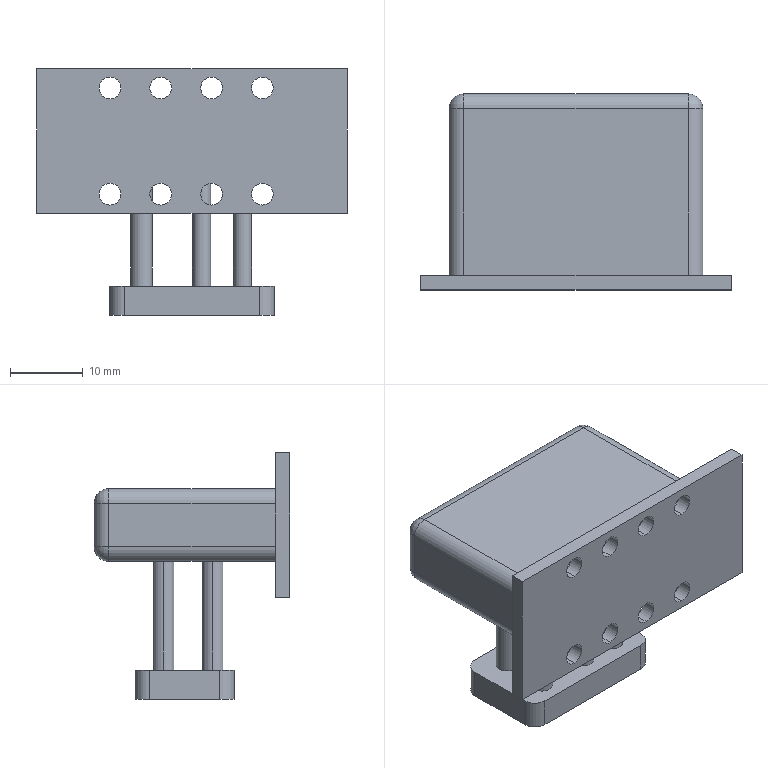Part | SolidWorks | features BaseBody 1 | 1 solid | 57 faces | box 42.805 x 27 x 33.95 mm | volume 11771 mm3 | cylinder 36 | plane 17 | sphere 4 | commonest cylinder face diameters 3 x20 4 x12 2.5 x4